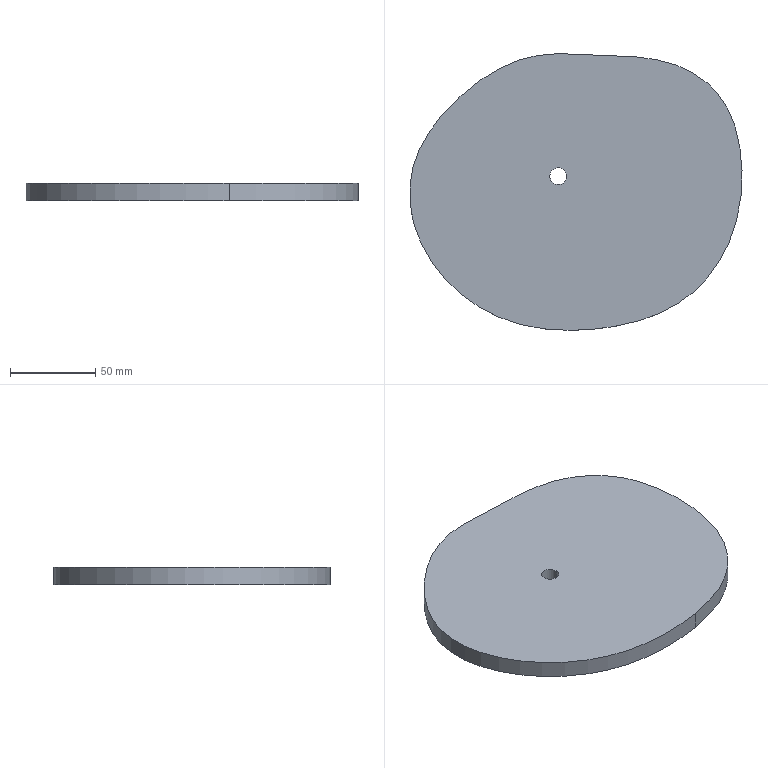Part | SolidWorks | features Extrusion 1 | 1 solid | 6 faces | box 194.935 x 162.289 x 10 mm | volume 255071 mm3 | cylinder 2 | plane 2 | spline 2 | commonest cylinder face diameters 10 x2
STEP:
#1=CARTESIAN_POINT('',(-5.,0.,10.));
#2=VERTEX_POINT('',#1);
#3=CARTESIAN_POINT('',(5.,0.,10.));
#4=VERTEX_POINT('',#3);
#5=CARTESIAN_POINT('',(0.,0.,10.));
#6=DIRECTION('',(0.,0.,1.));
#7=DIRECTION('',(1.,0.,0.));
#8=AXIS2_PLACEMENT_3D('',#5,#6,#7);
#9=CIRCLE('',#8,5.);
#10=EDGE_CURVE('',#2,#4,#9,.T.);
#11=ORIENTED_EDGE('',*,*,#10,.T.);
#12=CARTESIAN_POINT('',(5.,0.,0.));
#13=VERTEX_POINT('',#12);
#14=CARTESIAN_POINT('',(5.,0.,10.));
#15=DIRECTION('',(0.,0.,-1.));
#16=VECTOR('',#15,1000.);
#17=LINE('',#14,#16);
#18=EDGE_CURVE('',#4,#13,#17,.T.);
#19=ORIENTED_EDGE('',*,*,#18,.T.);
#20=CARTESIAN_POINT('',(-5.,0.,0.));
#21=VERTEX_POINT('',#20);
#22=CARTESIAN_POINT('',(0.,0.,0.));
#23=DIRECTION('',(0.,0.,1.));
#24=DIRECTION('',(1.,0.,0.));
#25=AXIS2_PLACEMENT_3D('',#22,#23,#24);
#26=CIRCLE('',#25,5.);
#27=EDGE_CURVE('',#21,#13,#26,.T.);
#28=ORIENTED_EDGE('',*,*,#27,.F.);
#29=CARTESIAN_POINT('',(-5.,0.,10.));
#30=DIRECTION('',(0.,0.,-1.));
#31=VECTOR('',#30,1000.);
#32=LINE('',#29,#31);
#33=EDGE_CURVE('',#2,#21,#32,.T.);
#34=ORIENTED_EDGE('',*,*,#33,.F.);
#35=EDGE_LOOP('',(#11,#19,#28,#34));
#36=FACE_OUTER_BOUND('',#35,.T.);
#37=CARTESIAN_POINT('',(0.,0.,10.));
#38=DIRECTION('',(0.,0.,-1.));
#39=DIRECTION('',(-1.,0.,0.));
#40=AXIS2_PLACEMENT_3D('',#37,#38,#39);
#41=CYLINDRICAL_SURFACE('',#40,5.);
#42=ADVANCED_FACE('',(#36),#41,.F.);
#43=CARTESIAN_POINT('',(32.099,-88.315,10.));
#44=VERTEX_POINT('',#43);
#45=CARTESIAN_POINT('',(0.,71.816,10.));
#46=VERTEX_POINT('',#45);
#47=CARTESIAN_POINT('',(32.099,-88.315,10.));
#48=CARTESIAN_POINT('',(39.092,-87.139,10.));
#49=CARTESIAN_POINT('',(52.353,-83.965,10.));
#50=CARTESIAN_POINT('',(70.582,-75.405,10.));
#51=CARTESIAN_POINT('',(87.006,-61.853,10.));
#52=CARTESIAN_POINT('',(99.872,-42.358,10.));
#53=CARTESIAN_POINT('',(106.776,-19.573,10.));
#54=CARTESIAN_POINT('',(108.259,1.416,10.));
#55=CARTESIAN_POINT('',(106.308,20.393,10.));
#56=CARTESIAN_POINT('',(101.146,38.709,10.));
#57=CARTESIAN_POINT('',(89.357,54.264,10.));
#58=CARTESIAN_POINT('',(73.202,64.366,10.));
#59=CARTESIAN_POINT('',(54.612,69.567,10.));
#60=CARTESIAN_POINT('',(35.352,70.648,10.));
#61=CARTESIAN_POINT('',(16.923,70.748,10.));
#62=CARTESIAN_POINT('',(5.531,71.943,10.));
#63=CARTESIAN_POINT('',(0.,71.816,10.));
#64=B_SPLINE_CURVE_WITH_KNOTS('',3,(#47,#48,#49,#50,#51,#52,#53,#54,#55,#56,#57,#58,#59,#60,#61,#62,#63),.UNSPECIFIED.,.F.,.F.,(4,1,1,1,1,1,1,1,1,1,1,1,1,1,4),(0.,21.305,40.809,60.047,84.633,109.876,130.833,147.498,167.135,187.311,204.563,223.578,244.718,262.399,279.04),.UNSPECIFIED.);
#65=EDGE_CURVE('',#44,#46,#64,.T.);
#66=ORIENTED_EDGE('',*,*,#65,.T.);
#67=CARTESIAN_POINT('',(0.,71.816,10.));
#68=CARTESIAN_POINT('',(-4.859,71.705,10.));
#69=CARTESIAN_POINT('',(-17.483,70.627,10.));
#70=CARTESIAN_POINT('',(-34.746,63.872,10.));
#71=CARTESIAN_POINT('',(-50.147,53.392,10.));
#72=CARTESIAN_POINT('',(-62.472,42.448,10.));
#73=CARTESIAN_POINT('',(-73.17,30.391,10.));
#74=CARTESIAN_POINT('',(-82.149,15.876,10.));
#75=CARTESIAN_POINT('',(-88.005,-2.656,10.));
#76=CARTESIAN_POINT('',(-86.927,-25.321,10.));
#77=CARTESIAN_POINT('',(-77.368,-47.678,10.));
#78=CARTESIAN_POINT('',(-60.946,-67.639,10.));
#79=CARTESIAN_POINT('',(-40.024,-81.711,10.));
#80=CARTESIAN_POINT('',(-15.273,-89.579,10.));
#81=CARTESIAN_POINT('',(8.555,-91.092,10.));
#82=CARTESIAN_POINT('',(24.79,-89.544,10.));
#83=CARTESIAN_POINT('',(32.099,-88.315,10.));
#84=B_SPLINE_CURVE_WITH_KNOTS('',3,(#67,#68,#69,#70,#71,#72,#73,#74,#75,#76,#77,#78,#79,#80,#81,#82,#83),.UNSPECIFIED.,.F.,.F.,(4,1,1,1,1,1,1,1,1,1,1,1,1,1,4),(279.04,293.657,316.906,333.763,349.53,366.375,382.074,400.552,423.972,448.648,472.41,500.88,523.123,549.806,572.073),.UNSPECIFIED.);
#85=EDGE_CURVE('',#46,#44,#84,.T.);
#86=ORIENTED_EDGE('',*,*,#85,.T.);
#87=EDGE_LOOP('',(#66,#86));
#88=FACE_OUTER_BOUND('',#87,.T.);
#89=ORIENTED_EDGE('',*,*,#10,.F.);
#90=CARTESIAN_POINT('',(0.,0.,10.));
#91=DIRECTION('',(0.,0.,1.));
#92=DIRECTION('',(1.,0.,0.));
#93=AXIS2_PLACEMENT_3D('',#90,#91,#92);
#94=CIRCLE('',#93,5.);
#95=EDGE_CURVE('',#4,#2,#94,.T.);
#96=ORIENTED_EDGE('',*,*,#95,.F.);
#97=EDGE_LOOP('',(#89,#96));
#98=FACE_BOUND('',#97,.T.);
#99=CARTESIAN_POINT('',(107.116,11.466,10.));
#100=DIRECTION('',(0.,0.,1.));
#101=DIRECTION('',(1.,0.,0.));
#102=AXIS2_PLACEMENT_3D('',#99,#100,#101);
#103=PLANE('',#102);
#104=ADVANCED_FACE('',(#88,#98),#103,.T.);
#105=CARTESIAN_POINT('',(32.099,-88.315,0.));
#106=VERTEX_POINT('',#105);
#107=CARTESIAN_POINT('',(0.,71.816,0.));
#108=VERTEX_POINT('',#107);
#109=CARTESIAN_POINT('',(32.099,-88.315,0.));
#110=CARTESIAN_POINT('',(39.092,-87.139,0.));
#111=CARTESIAN_POINT('',(52.353,-83.965,0.));
#112=CARTESIAN_POINT('',(70.582,-75.405,0.));
#113=CARTESIAN_POINT('',(87.006,-61.853,0.));
#114=CARTESIAN_POINT('',(99.872,-42.358,0.));
#115=CARTESIAN_POINT('',(106.776,-19.573,0.));
#116=CARTESIAN_POINT('',(108.259,1.416,0.));
#117=CARTESIAN_POINT('',(106.308,20.393,0.));
#118=CARTESIAN_POINT('',(101.146,38.709,0.));
#119=CARTESIAN_POINT('',(89.357,54.264,0.));
#120=CARTESIAN_POINT('',(73.202,64.366,0.));
#121=CARTESIAN_POINT('',(54.612,69.567,0.));
#122=CARTESIAN_POINT('',(35.352,70.648,0.));
#123=CARTESIAN_POINT('',(16.923,70.748,0.));
#124=CARTESIAN_POINT('',(5.531,71.943,0.));
#125=CARTESIAN_POINT('',(0.,71.816,0.));
#126=B_SPLINE_CURVE_WITH_KNOTS('',3,(#109,#110,#111,#112,#113,#114,#115,#116,#117,#118,#119,#120,#121,#122,#123,#124,#125),.UNSPECIFIED.,.F.,.F.,(4,1,1,1,1,1,1,1,1,1,1,1,1,1,4),(0.,21.305,40.809,60.047,84.633,109.876,130.833,147.498,167.135,187.311,204.563,223.578,244.718,262.399,279.04),.UNSPECIFIED.);
#127=EDGE_CURVE('',#106,#108,#126,.T.);
#128=ORIENTED_EDGE('',*,*,#127,.F.);
#129=CARTESIAN_POINT('',(0.,71.816,0.));
#130=CARTESIAN_POINT('',(-4.859,71.705,0.));
#131=CARTESIAN_POINT('',(-17.483,70.627,0.));
#132=CARTESIAN_POINT('',(-34.746,63.872,0.));
#133=CARTESIAN_POINT('',(-50.147,53.392,0.));
#134=CARTESIAN_POINT('',(-62.472,42.448,0.));
#135=CARTESIAN_POINT('',(-73.17,30.391,0.));
#136=CARTESIAN_POINT('',(-82.149,15.876,0.));
#137=CARTESIAN_POINT('',(-88.005,-2.656,0.));
#138=CARTESIAN_POINT('',(-86.927,-25.321,0.));
#139=CARTESIAN_POINT('',(-77.368,-47.678,0.));
#140=CARTESIAN_POINT('',(-60.946,-67.639,0.));
#141=CARTESIAN_POINT('',(-40.024,-81.711,0.));
#142=CARTESIAN_POINT('',(-15.273,-89.579,0.));
#143=CARTESIAN_POINT('',(8.555,-91.092,0.));
#144=CARTESIAN_POINT('',(24.79,-89.544,0.));
#145=CARTESIAN_POINT('',(32.099,-88.315,0.));
#146=B_SPLINE_CURVE_WITH_KNOTS('',3,(#129,#130,#131,#132,#133,#134,#135,#136,#137,#138,#139,#140,#141,#142,#143,#144,#145),.UNSPECIFIED.,.F.,.F.,(4,1,1,1,1,1,1,1,1,1,1,1,1,1,4),(279.04,293.657,316.906,333.763,349.53,366.375,382.074,400.552,423.972,448.648,472.41,500.88,523.123,549.806,572.073),.UNSPECIFIED.);
#147=EDGE_CURVE('',#108,#106,#146,.T.);
#148=ORIENTED_EDGE('',*,*,#147,.F.);
#149=EDGE_LOOP('',(#128,#148));
#150=FACE_OUTER_BOUND('',#149,.T.);
#151=ORIENTED_EDGE('',*,*,#27,.T.);
#152=CARTESIAN_POINT('',(0.,0.,0.));
#153=DIRECTION('',(0.,0.,1.));
#154=DIRECTION('',(1.,0.,0.));
#155=AXIS2_PLACEMENT_3D('',#152,#153,#154);
#156=CIRCLE('',#155,5.);
#157=EDGE_CURVE('',#13,#21,#156,.T.);
#158=ORIENTED_EDGE('',*,*,#157,.T.);
#159=EDGE_LOOP('',(#151,#158));
#160=FACE_BOUND('',#159,.T.);
#161=CARTESIAN_POINT('',(107.116,11.466,0.));
#162=DIRECTION('',(0.,0.,1.));
#163=DIRECTION('',(1.,0.,0.));
#164=AXIS2_PLACEMENT_3D('',#161,#162,#163);
#165=PLANE('',#164);
#166=ADVANCED_FACE('',(#150,#160),#165,.F.);
#167=ORIENTED_EDGE('',*,*,#127,.T.);
#168=CARTESIAN_POINT('',(0.,71.816,10.));
#169=DIRECTION('',(0.,0.,-1.));
#170=VECTOR('',#169,1000.);
#171=LINE('',#168,#170);
#172=EDGE_CURVE('',#46,#108,#171,.T.);
#173=ORIENTED_EDGE('',*,*,#172,.F.);
#174=ORIENTED_EDGE('',*,*,#65,.F.);
#175=CARTESIAN_POINT('',(32.099,-88.315,10.));
#176=DIRECTION('',(0.,0.,-1.));
#177=VECTOR('',#176,1000.);
#178=LINE('',#175,#177);
#179=EDGE_CURVE('',#44,#106,#178,.T.);
#180=ORIENTED_EDGE('',*,*,#179,.T.);
#181=EDGE_LOOP('',(#167,#173,#174,#180));
#182=FACE_OUTER_BOUND('',#181,.T.);
#183=CARTESIAN_POINT('',(32.099,-88.315,10.));
#184=CARTESIAN_POINT('',(32.099,-88.315,0.));
#185=CARTESIAN_POINT('',(39.092,-87.139,10.));
#186=CARTESIAN_POINT('',(39.092,-87.139,0.));
#187=CARTESIAN_POINT('',(52.353,-83.965,10.));
#188=CARTESIAN_POINT('',(52.353,-83.965,0.));
#189=CARTESIAN_POINT('',(70.582,-75.405,10.));
#190=CARTESIAN_POINT('',(70.582,-75.405,0.));
#191=CARTESIAN_POINT('',(87.006,-61.853,10.));
#192=CARTESIAN_POINT('',(87.006,-61.853,0.));
#193=CARTESIAN_POINT('',(99.872,-42.358,10.));
#194=CARTESIAN_POINT('',(99.872,-42.358,0.));
#195=CARTESIAN_POINT('',(106.776,-19.573,10.));
#196=CARTESIAN_POINT('',(106.776,-19.573,0.));
#197=CARTESIAN_POINT('',(108.259,1.416,10.));
#198=CARTESIAN_POINT('',(108.259,1.416,0.));
#199=CARTESIAN_POINT('',(106.308,20.393,10.));
#200=CARTESIAN_POINT('',(106.308,20.393,0.));
#201=CARTESIAN_POINT('',(101.146,38.709,10.));
#202=CARTESIAN_POINT('',(101.146,38.709,0.));
#203=CARTESIAN_POINT('',(89.357,54.264,10.));
#204=CARTESIAN_POINT('',(89.357,54.264,0.));
#205=CARTESIAN_POINT('',(73.202,64.366,10.));
#206=CARTESIAN_POINT('',(73.202,64.366,0.));
#207=CARTESIAN_POINT('',(54.612,69.567,10.));
#208=CARTESIAN_POINT('',(54.612,69.567,0.));
#209=CARTESIAN_POINT('',(35.352,70.648,10.));
#210=CARTESIAN_POINT('',(35.352,70.648,0.));
#211=CARTESIAN_POINT('',(16.923,70.748,10.));
#212=CARTESIAN_POINT('',(16.923,70.748,0.));
#213=CARTESIAN_POINT('',(5.531,71.943,10.));
#214=CARTESIAN_POINT('',(5.531,71.943,0.));
#215=CARTESIAN_POINT('',(-0.000000016,71.816,10.));
#216=CARTESIAN_POINT('',(-0.000000016,71.816,0.));
#217=B_SPLINE_SURFACE_WITH_KNOTS('',3,1,((#183,#184),(#185,#186),(#187,#188),(#189,#190),(#191,#192),(#193,#194),(#195,#196),(#197,#198),(#199,#200),(#201,#202),(#203,#204),(#205,#206),(#207,#208),(#209,#210),(#211,#212),(#213,#214),(#215,#216)),.UNSPECIFIED.,.F.,.F.,.F.,(4,1,1,1,1,1,1,1,1,1,1,1,1,1,4),(2,2),(0.,21.305,40.809,60.047,84.633,109.876,130.833,147.498,167.135,187.311,204.563,223.578,244.718,262.399,279.04),(0.,1.),.UNSPECIFIED.);
#218=ADVANCED_FACE('',(#182),#217,.F.);
#219=ORIENTED_EDGE('',*,*,#147,.T.);
#220=ORIENTED_EDGE('',*,*,#179,.F.);
#221=ORIENTED_EDGE('',*,*,#85,.F.);
#222=ORIENTED_EDGE('',*,*,#172,.T.);
#223=EDGE_LOOP('',(#219,#220,#221,#222));
#224=FACE_OUTER_BOUND('',#223,.T.);
#225=CARTESIAN_POINT('',(0.,71.816,10.));
#226=CARTESIAN_POINT('',(0.,71.816,0.));
#227=CARTESIAN_POINT('',(-4.859,71.705,10.));
#228=CARTESIAN_POINT('',(-4.859,71.705,0.));
#229=CARTESIAN_POINT('',(-17.483,70.627,10.));
#230=CARTESIAN_POINT('',(-17.483,70.627,0.));
#231=CARTESIAN_POINT('',(-34.746,63.872,10.));
#232=CARTESIAN_POINT('',(-34.746,63.872,0.));
#233=CARTESIAN_POINT('',(-50.147,53.392,10.));
#234=CARTESIAN_POINT('',(-50.147,53.392,0.));
#235=CARTESIAN_POINT('',(-62.472,42.448,10.));
#236=CARTESIAN_POINT('',(-62.472,42.448,0.));
#237=CARTESIAN_POINT('',(-73.17,30.391,10.));
#238=CARTESIAN_POINT('',(-73.17,30.391,0.));
#239=CARTESIAN_POINT('',(-82.149,15.876,10.));
#240=CARTESIAN_POINT('',(-82.149,15.876,0.));
#241=CARTESIAN_POINT('',(-88.005,-2.656,10.));
#242=CARTESIAN_POINT('',(-88.005,-2.656,0.));
#243=CARTESIAN_POINT('',(-86.927,-25.321,10.));
#244=CARTESIAN_POINT('',(-86.927,-25.321,0.));
#245=CARTESIAN_POINT('',(-77.368,-47.678,10.));
#246=CARTESIAN_POINT('',(-77.368,-47.678,0.));
#247=CARTESIAN_POINT('',(-60.946,-67.639,10.));
#248=CARTESIAN_POINT('',(-60.946,-67.639,0.));
#249=CARTESIAN_POINT('',(-40.024,-81.711,10.));
#250=CARTESIAN_POINT('',(-40.024,-81.711,0.));
#251=CARTESIAN_POINT('',(-15.273,-89.579,10.));
#252=CARTESIAN_POINT('',(-15.273,-89.579,0.));
#253=CARTESIAN_POINT('',(8.555,-91.092,10.));
#254=CARTESIAN_POINT('',(8.555,-91.092,0.));
#255=CARTESIAN_POINT('',(24.79,-89.544,10.));
#256=CARTESIAN_POINT('',(24.79,-89.544,0.));
#257=CARTESIAN_POINT('',(32.099,-88.315,10.));
#258=CARTESIAN_POINT('',(32.099,-88.315,0.));
#259=B_SPLINE_SURFACE_WITH_KNOTS('',3,1,((#225,#226),(#227,#228),(#229,#230),(#231,#232),(#233,#234),(#235,#236),(#237,#238),(#239,#240),(#241,#242),(#243,#244),(#245,#246),(#247,#248),(#249,#250),(#251,#252),(#253,#254),(#255,#256),(#257,#258)),.UNSPECIFIED.,.F.,.F.,.F.,(4,1,1,1,1,1,1,1,1,1,1,1,1,1,4),(2,2),(279.04,293.657,316.906,333.763,349.53,366.375,382.074,400.552,423.972,448.648,472.41,500.88,523.123,549.806,572.073),(0.,1.),.UNSPECIFIED.);
#260=ADVANCED_FACE('',(#224),#259,.F.);
#261=ORIENTED_EDGE('',*,*,#18,.F.);
#262=ORIENTED_EDGE('',*,*,#95,.T.);
#263=ORIENTED_EDGE('',*,*,#33,.T.);
#264=ORIENTED_EDGE('',*,*,#157,.F.);
#265=EDGE_LOOP('',(#261,#262,#263,#264));
#266=FACE_OUTER_BOUND('',#265,.T.);
#267=CARTESIAN_POINT('',(0.,0.,10.));
#268=DIRECTION('',(0.,0.,-1.));
#269=DIRECTION('',(-1.,0.,0.));
#270=AXIS2_PLACEMENT_3D('',#267,#268,#269);
#271=CYLINDRICAL_SURFACE('',#270,5.);
#272=ADVANCED_FACE('',(#266),#271,.F.);
#273=CLOSED_SHELL('',(#42,#104,#166,#218,#260,#272));
#274=MANIFOLD_SOLID_BREP('',#273);
#275=CARTESIAN_POINT('',(0.,0.,0.));
#276=DIRECTION('',(0.,0.,1.));
#277=DIRECTION('',(1.,0.,0.));
#278=AXIS2_PLACEMENT_3D('',#275,#276,#277);
#279=(LENGTH_UNIT()NAMED_UNIT(*)SI_UNIT(.MILLI.,.METRE.));
#280=UNCERTAINTY_MEASURE_WITH_UNIT(LENGTH_MEASURE(0.00001),#279,'','');
#281=(NAMED_UNIT(*)PLANE_ANGLE_UNIT()SI_UNIT($,.RADIAN.));
#282=(NAMED_UNIT(*)SI_UNIT($,.STERADIAN.)SOLID_ANGLE_UNIT());
#283=(GEOMETRIC_REPRESENTATION_CONTEXT(3)GLOBAL_UNCERTAINTY_ASSIGNED_CONTEXT((#280))GLOBAL_UNIT_ASSIGNED_CONTEXT((#279,#281,#282))REPRESENTATION_CONTEXT('',''));
#284=ADVANCED_BREP_SHAPE_REPRESENTATION('',(#274,#278),#283);